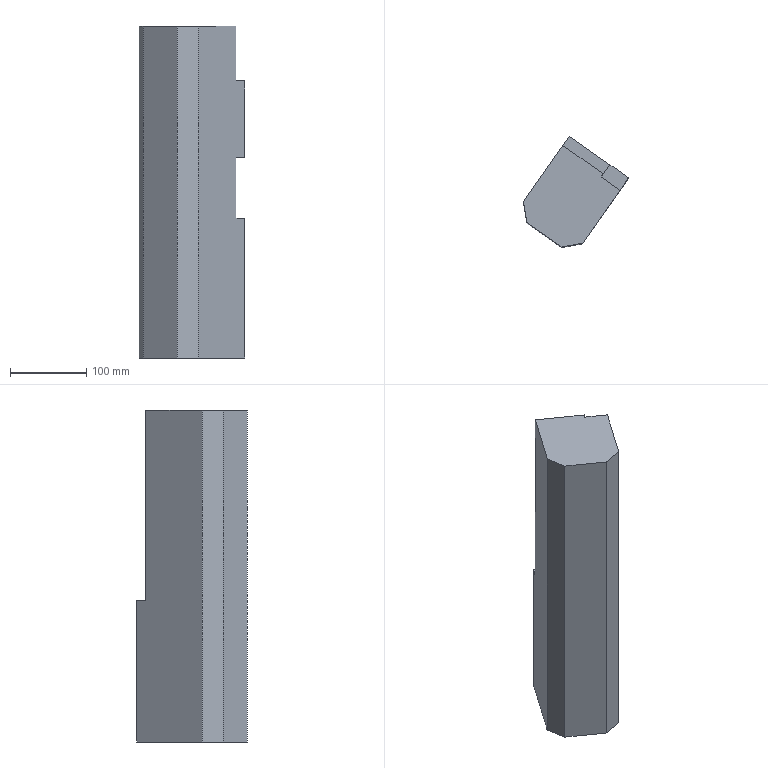Part | NX | features solid 2 | 1 solid | 19 faces | box 138.045 x 145.412 x 435 mm | volume 4656663 mm3 | plane 19
STEP:
#1=CARTESIAN_POINT('',(-261.776,-225.662,-154.062));
#2=VERTEX_POINT('',#1);
#3=CARTESIAN_POINT('',(-216.723,-257.209,-154.062));
#4=VERTEX_POINT('',#3);
#5=CARTESIAN_POINT('',(-278.159,-214.19,-154.062));
#6=DIRECTION('',(0.8192,-0.5736,0.));
#7=VECTOR('',#6,1000.);
#8=LINE('',#5,#7);
#9=EDGE_CURVE('',#2,#4,#8,.T.);
#10=ORIENTED_EDGE('',*,*,#9,.T.);
#11=CARTESIAN_POINT('',(-188.868,-252.297,-154.062));
#12=VERTEX_POINT('',#11);
#13=CARTESIAN_POINT('',(-188.868,-252.297,-154.062));
#14=DIRECTION('',(0.9848,0.1736,0.));
#15=VECTOR('',#14,1000.);
#16=LINE('',#13,#15);
#17=EDGE_CURVE('',#4,#12,#16,.T.);
#18=ORIENTED_EDGE('',*,*,#17,.T.);
#19=CARTESIAN_POINT('',(-140.114,-182.669,-154.062));
#20=VERTEX_POINT('',#19);
#21=CARTESIAN_POINT('',(-48.342,-51.605,-154.062));
#22=DIRECTION('',(0.5736,0.8192,0.));
#23=VECTOR('',#22,1000.);
#24=LINE('',#21,#23);
#25=EDGE_CURVE('',#20,#12,#24,.F.);
#26=ORIENTED_EDGE('',*,*,#25,.F.);
#27=CARTESIAN_POINT('',(-164.689,-165.462,-154.062));
#28=VERTEX_POINT('',#27);
#29=CARTESIAN_POINT('',(-217.934,-128.179,-154.062));
#30=DIRECTION('',(0.8192,-0.5736,0.));
#31=VECTOR('',#30,1000.);
#32=LINE('',#29,#31);
#33=EDGE_CURVE('',#28,#20,#32,.T.);
#34=ORIENTED_EDGE('',*,*,#33,.F.);
#35=CARTESIAN_POINT('',(-161.821,-161.366,-154.062));
#36=VERTEX_POINT('',#35);
#37=CARTESIAN_POINT('',(-161.821,-161.366,-154.062));
#38=DIRECTION('',(0.5736,0.8192,0.));
#39=VECTOR('',#38,1000.);
#40=LINE('',#37,#39);
#41=EDGE_CURVE('',#28,#36,#40,.T.);
#42=ORIENTED_EDGE('',*,*,#41,.T.);
#43=CARTESIAN_POINT('',(-215.066,-124.084,-154.062));
#44=VERTEX_POINT('',#43);
#45=CARTESIAN_POINT('',(-215.066,-124.084,-154.062));
#46=DIRECTION('',(0.8192,-0.5736,0.));
#47=VECTOR('',#46,1000.);
#48=LINE('',#45,#47);
#49=EDGE_CURVE('',#44,#36,#48,.T.);
#50=ORIENTED_EDGE('',*,*,#49,.F.);
#51=CARTESIAN_POINT('',(-266.688,-197.807,-154.062));
#52=VERTEX_POINT('',#51);
#53=CARTESIAN_POINT('',(-215.066,-124.084,-154.062));
#54=DIRECTION('',(-0.5736,-0.8192,0.));
#55=VECTOR('',#54,1000.);
#56=LINE('',#53,#55);
#57=EDGE_CURVE('',#44,#52,#56,.T.);
#58=ORIENTED_EDGE('',*,*,#57,.T.);
#59=CARTESIAN_POINT('',(-261.776,-225.662,-154.062));
#60=DIRECTION('',(0.1736,-0.9848,0.));
#61=VECTOR('',#60,1000.);
#62=LINE('',#59,#61);
#63=EDGE_CURVE('',#52,#2,#62,.T.);
#64=ORIENTED_EDGE('',*,*,#63,.T.);
#65=EDGE_LOOP('',(#10,#18,#26,#34,#42,#50,#58,#64));
#66=FACE_BOUND('',#65,.T.);
#67=CARTESIAN_POINT('',(-215.066,-124.084,-154.062));
#68=DIRECTION('',(0.,0.,-1.));
#69=DIRECTION('',(-0.5736,-0.8192,0.));
#70=AXIS2_PLACEMENT_3D('',#67,#68,#69);
#71=PLANE('',#70);
#72=ADVANCED_FACE('',(#66),#71,.F.);
#73=CARTESIAN_POINT('',(-161.821,-161.366,-226.082));
#74=VERTEX_POINT('',#73);
#75=CARTESIAN_POINT('',(-161.821,-161.366,-326.082));
#76=VERTEX_POINT('',#75);
#77=CARTESIAN_POINT('',(-161.821,-161.366,-401.082));
#78=DIRECTION('',(0.,0.,-1.));
#79=VECTOR('',#78,1000.);
#80=LINE('',#77,#79);
#81=EDGE_CURVE('',#74,#76,#80,.T.);
#82=ORIENTED_EDGE('',*,*,#81,.T.);
#83=CARTESIAN_POINT('',(-161.821,-161.366,-404.062));
#84=VERTEX_POINT('',#83);
#85=CARTESIAN_POINT('',(-161.821,-161.366,-401.082));
#86=DIRECTION('',(0.,0.,-1.));
#87=VECTOR('',#86,1000.);
#88=LINE('',#85,#87);
#89=EDGE_CURVE('',#76,#84,#88,.T.);
#90=ORIENTED_EDGE('',*,*,#89,.T.);
#91=CARTESIAN_POINT('',(-215.066,-124.084,-404.062));
#92=VERTEX_POINT('',#91);
#93=CARTESIAN_POINT('',(-215.066,-124.084,-404.062));
#94=DIRECTION('',(-0.8192,0.5736,0.));
#95=VECTOR('',#94,1000.);
#96=LINE('',#93,#95);
#97=EDGE_CURVE('',#84,#92,#96,.T.);
#98=ORIENTED_EDGE('',*,*,#97,.T.);
#99=CARTESIAN_POINT('',(-215.066,-124.084,-401.082));
#100=DIRECTION('',(0.,0.,-1.));
#101=VECTOR('',#100,1000.);
#102=LINE('',#99,#101);
#103=EDGE_CURVE('',#44,#92,#102,.T.);
#104=ORIENTED_EDGE('',*,*,#103,.F.);
#105=ORIENTED_EDGE('',*,*,#49,.T.);
#106=CARTESIAN_POINT('',(-161.821,-161.366,-401.082));
#107=DIRECTION('',(0.,0.,1.));
#108=VECTOR('',#107,1000.);
#109=LINE('',#106,#108);
#110=EDGE_CURVE('',#74,#36,#109,.T.);
#111=ORIENTED_EDGE('',*,*,#110,.F.);
#112=EDGE_LOOP('',(#82,#90,#98,#104,#105,#111));
#113=FACE_BOUND('',#112,.T.);
#114=CARTESIAN_POINT('',(-215.066,-124.084,-401.082));
#115=DIRECTION('',(-0.5736,-0.8192,0.));
#116=DIRECTION('',(0.8192,-0.5736,0.));
#117=AXIS2_PLACEMENT_3D('',#114,#115,#116);
#118=PLANE('',#117);
#119=ADVANCED_FACE('',(#113),#118,.F.);
#120=CARTESIAN_POINT('',(-153.217,-149.079,-404.062));
#121=VERTEX_POINT('',#120);
#122=CARTESIAN_POINT('',(-153.217,-149.079,-406.082));
#123=VERTEX_POINT('',#122);
#124=CARTESIAN_POINT('',(-153.217,-149.079,-326.082));
#125=DIRECTION('',(0.,0.,-1.));
#126=VECTOR('',#125,1000.);
#127=LINE('',#124,#126);
#128=EDGE_CURVE('',#121,#123,#127,.T.);
#129=ORIENTED_EDGE('',*,*,#128,.T.);
#130=CARTESIAN_POINT('',(-128.643,-166.286,-406.082));
#131=VERTEX_POINT('',#130);
#132=CARTESIAN_POINT('',(-153.217,-149.079,-406.082));
#133=DIRECTION('',(0.8192,-0.5736,0.));
#134=VECTOR('',#133,1000.);
#135=LINE('',#132,#134);
#136=EDGE_CURVE('',#123,#131,#135,.T.);
#137=ORIENTED_EDGE('',*,*,#136,.T.);
#138=CARTESIAN_POINT('',(-128.643,-166.286,-589.062));
#139=VERTEX_POINT('',#138);
#140=CARTESIAN_POINT('',(-128.643,-166.286,-400.));
#141=DIRECTION('',(0.,0.,1.));
#142=VECTOR('',#141,1000.);
#143=LINE('',#140,#142);
#144=EDGE_CURVE('',#131,#139,#143,.F.);
#145=ORIENTED_EDGE('',*,*,#144,.T.);
#146=CARTESIAN_POINT('',(-206.462,-111.796,-589.062));
#147=VERTEX_POINT('',#146);
#148=CARTESIAN_POINT('',(-206.544,-111.739,-589.062));
#149=DIRECTION('',(0.8192,-0.5736,0.));
#150=VECTOR('',#149,1000.);
#151=LINE('',#148,#150);
#152=EDGE_CURVE('',#139,#147,#151,.F.);
#153=ORIENTED_EDGE('',*,*,#152,.T.);
#154=CARTESIAN_POINT('',(-206.462,-111.796,-404.062));
#155=VERTEX_POINT('',#154);
#156=CARTESIAN_POINT('',(-206.462,-111.796,-401.082));
#157=DIRECTION('',(0.,0.,-1.));
#158=VECTOR('',#157,1000.);
#159=LINE('',#156,#158);
#160=EDGE_CURVE('',#155,#147,#159,.T.);
#161=ORIENTED_EDGE('',*,*,#160,.F.);
#162=CARTESIAN_POINT('',(-153.217,-149.079,-404.062));
#163=DIRECTION('',(-0.8192,0.5736,0.));
#164=VECTOR('',#163,1000.);
#165=LINE('',#162,#164);
#166=EDGE_CURVE('',#121,#155,#165,.T.);
#167=ORIENTED_EDGE('',*,*,#166,.F.);
#168=EDGE_LOOP('',(#129,#137,#145,#153,#161,#167));
#169=FACE_BOUND('',#168,.T.);
#170=CARTESIAN_POINT('',(-153.217,-149.079,-461.082));
#171=DIRECTION('',(0.5736,0.8192,0.));
#172=DIRECTION('',(-0.8192,0.5736,0.));
#173=AXIS2_PLACEMENT_3D('',#170,#171,#172);
#174=PLANE('',#173);
#175=ADVANCED_FACE('',(#169),#174,.T.);
#176=CARTESIAN_POINT('',(-188.868,-252.297,-589.062));
#177=VERTEX_POINT('',#176);
#178=CARTESIAN_POINT('',(-197.472,-264.584,-589.062));
#179=DIRECTION('',(-0.5736,-0.8192,0.));
#180=VECTOR('',#179,1000.);
#181=LINE('',#178,#180);
#182=EDGE_CURVE('',#139,#177,#181,.T.);
#183=ORIENTED_EDGE('',*,*,#182,.T.);
#184=CARTESIAN_POINT('',(-216.723,-257.209,-589.062));
#185=VERTEX_POINT('',#184);
#186=CARTESIAN_POINT('',(-188.868,-252.297,-589.062));
#187=DIRECTION('',(0.9848,0.1736,0.));
#188=VECTOR('',#187,1000.);
#189=LINE('',#186,#188);
#190=EDGE_CURVE('',#177,#185,#189,.F.);
#191=ORIENTED_EDGE('',*,*,#190,.T.);
#192=CARTESIAN_POINT('',(-261.776,-225.662,-589.062));
#193=VERTEX_POINT('',#192);
#194=CARTESIAN_POINT('',(-278.241,-214.133,-589.062));
#195=DIRECTION('',(0.8192,-0.5736,0.));
#196=VECTOR('',#195,1000.);
#197=LINE('',#194,#196);
#198=EDGE_CURVE('',#185,#193,#197,.F.);
#199=ORIENTED_EDGE('',*,*,#198,.T.);
#200=CARTESIAN_POINT('',(-266.688,-197.807,-589.062));
#201=VERTEX_POINT('',#200);
#202=CARTESIAN_POINT('',(-261.776,-225.662,-589.062));
#203=DIRECTION('',(0.1736,-0.9848,0.));
#204=VECTOR('',#203,1000.);
#205=LINE('',#202,#204);
#206=EDGE_CURVE('',#193,#201,#205,.F.);
#207=ORIENTED_EDGE('',*,*,#206,.T.);
#208=CARTESIAN_POINT('',(-275.291,-210.095,-589.062));
#209=DIRECTION('',(0.5736,0.8192,0.));
#210=VECTOR('',#209,1000.);
#211=LINE('',#208,#210);
#212=EDGE_CURVE('',#147,#201,#211,.F.);
#213=ORIENTED_EDGE('',*,*,#212,.F.);
#214=ORIENTED_EDGE('',*,*,#152,.F.);
#215=EDGE_LOOP('',(#183,#191,#199,#207,#213,#214));
#216=FACE_BOUND('',#215,.T.);
#217=CARTESIAN_POINT('',(-275.373,-210.037,-589.062));
#218=DIRECTION('',(0.,0.,-1.));
#219=DIRECTION('',(0.5736,0.8192,0.));
#220=AXIS2_PLACEMENT_3D('',#217,#218,#219);
#221=PLANE('',#220);
#222=ADVANCED_FACE('',(#216),#221,.T.);
#223=ORIENTED_EDGE('',*,*,#212,.T.);
#224=CARTESIAN_POINT('',(-266.688,-197.807,-151.082));
#225=DIRECTION('',(0.,0.,1.));
#226=VECTOR('',#225,1000.);
#227=LINE('',#224,#226);
#228=EDGE_CURVE('',#201,#52,#227,.T.);
#229=ORIENTED_EDGE('',*,*,#228,.T.);
#230=ORIENTED_EDGE('',*,*,#57,.F.);
#231=ORIENTED_EDGE('',*,*,#103,.T.);
#232=CARTESIAN_POINT('',(-215.066,-124.084,-404.062));
#233=DIRECTION('',(-0.5736,-0.8192,0.));
#234=VECTOR('',#233,1000.);
#235=LINE('',#232,#234);
#236=EDGE_CURVE('',#155,#92,#235,.T.);
#237=ORIENTED_EDGE('',*,*,#236,.F.);
#238=ORIENTED_EDGE('',*,*,#160,.T.);
#239=EDGE_LOOP('',(#223,#229,#230,#231,#237,#238));
#240=FACE_BOUND('',#239,.T.);
#241=CARTESIAN_POINT('',(-215.066,-124.084,-151.082));
#242=DIRECTION('',(-0.8192,0.5736,0.));
#243=DIRECTION('',(-0.5736,-0.8192,0.));
#244=AXIS2_PLACEMENT_3D('',#241,#242,#243);
#245=PLANE('',#244);
#246=ADVANCED_FACE('',(#240),#245,.T.);
#247=ORIENTED_EDGE('',*,*,#198,.F.);
#248=CARTESIAN_POINT('',(-216.723,-257.209,-192.696));
#249=DIRECTION('',(0.,0.,1.));
#250=VECTOR('',#249,1000.);
#251=LINE('',#248,#250);
#252=EDGE_CURVE('',#185,#4,#251,.T.);
#253=ORIENTED_EDGE('',*,*,#252,.T.);
#254=ORIENTED_EDGE('',*,*,#9,.F.);
#255=CARTESIAN_POINT('',(-261.776,-225.662,-589.062));
#256=DIRECTION('',(0.,0.,-1.));
#257=VECTOR('',#256,1000.);
#258=LINE('',#255,#257);
#259=EDGE_CURVE('',#2,#193,#258,.T.);
#260=ORIENTED_EDGE('',*,*,#259,.T.);
#261=EDGE_LOOP('',(#247,#253,#254,#260));
#262=FACE_BOUND('',#261,.T.);
#263=CARTESIAN_POINT('',(-789.915,144.145,-192.696));
#264=DIRECTION('',(0.5736,0.8192,0.));
#265=DIRECTION('',(-0.8192,0.5736,0.));
#266=AXIS2_PLACEMENT_3D('',#263,#264,#265);
#267=PLANE('',#266);
#268=ADVANCED_FACE('',(#262),#267,.F.);
#269=CARTESIAN_POINT('',(-161.821,-161.366,-404.062));
#270=DIRECTION('',(-0.5736,-0.8192,0.));
#271=VECTOR('',#270,1000.);
#272=LINE('',#269,#271);
#273=EDGE_CURVE('',#121,#84,#272,.T.);
#274=ORIENTED_EDGE('',*,*,#273,.F.);
#275=ORIENTED_EDGE('',*,*,#166,.T.);
#276=ORIENTED_EDGE('',*,*,#236,.T.);
#277=ORIENTED_EDGE('',*,*,#97,.F.);
#278=EDGE_LOOP('',(#274,#275,#276,#277));
#279=FACE_BOUND('',#278,.T.);
#280=CARTESIAN_POINT('',(-161.821,-161.366,-404.062));
#281=DIRECTION('',(0.,0.,1.));
#282=DIRECTION('',(0.5736,0.8192,0.));
#283=AXIS2_PLACEMENT_3D('',#280,#281,#282);
#284=PLANE('',#283);
#285=ADVANCED_FACE('',(#279),#284,.T.);
#286=CARTESIAN_POINT('',(-140.114,-182.669,-326.082));
#287=VERTEX_POINT('',#286);
#288=CARTESIAN_POINT('',(-128.643,-166.286,-326.082));
#289=VERTEX_POINT('',#288);
#290=CARTESIAN_POINT('',(-137.246,-178.573,-326.082));
#291=DIRECTION('',(-0.5736,-0.8192,0.));
#292=VECTOR('',#291,1000.);
#293=LINE('',#290,#292);
#294=EDGE_CURVE('',#287,#289,#293,.F.);
#295=ORIENTED_EDGE('',*,*,#294,.F.);
#296=CARTESIAN_POINT('',(-164.689,-165.462,-326.082));
#297=VERTEX_POINT('',#296);
#298=CARTESIAN_POINT('',(-164.689,-165.462,-326.082));
#299=DIRECTION('',(0.8192,-0.5736,0.));
#300=VECTOR('',#299,1000.);
#301=LINE('',#298,#300);
#302=EDGE_CURVE('',#297,#287,#301,.T.);
#303=ORIENTED_EDGE('',*,*,#302,.F.);
#304=CARTESIAN_POINT('',(-161.821,-161.366,-326.082));
#305=DIRECTION('',(0.5736,0.8192,0.));
#306=VECTOR('',#305,1000.);
#307=LINE('',#304,#306);
#308=EDGE_CURVE('',#297,#76,#307,.T.);
#309=ORIENTED_EDGE('',*,*,#308,.T.);
#310=CARTESIAN_POINT('',(-153.217,-149.079,-326.082));
#311=VERTEX_POINT('',#310);
#312=CARTESIAN_POINT('',(-161.821,-161.366,-326.082));
#313=DIRECTION('',(0.5736,0.8192,0.));
#314=VECTOR('',#313,1000.);
#315=LINE('',#312,#314);
#316=EDGE_CURVE('',#76,#311,#315,.T.);
#317=ORIENTED_EDGE('',*,*,#316,.T.);
#318=CARTESIAN_POINT('',(-153.217,-149.079,-326.082));
#319=DIRECTION('',(-0.8192,0.5736,0.));
#320=VECTOR('',#319,1000.);
#321=LINE('',#318,#320);
#322=EDGE_CURVE('',#311,#289,#321,.F.);
#323=ORIENTED_EDGE('',*,*,#322,.T.);
#324=EDGE_LOOP('',(#295,#303,#309,#317,#323));
#325=FACE_BOUND('',#324,.T.);
#326=CARTESIAN_POINT('',(-161.821,-161.366,-326.082));
#327=DIRECTION('',(0.,0.,-1.));
#328=DIRECTION('',(-0.9063,-0.4226,0.));
#329=AXIS2_PLACEMENT_3D('',#326,#327,#328);
#330=PLANE('',#329);
#331=ADVANCED_FACE('',(#325),#330,.T.);
#332=CARTESIAN_POINT('',(-164.689,-165.462,-226.082));
#333=VERTEX_POINT('',#332);
#334=CARTESIAN_POINT('',(-140.114,-182.669,-226.082));
#335=VERTEX_POINT('',#334);
#336=CARTESIAN_POINT('',(-217.934,-128.179,-226.082));
#337=DIRECTION('',(0.8192,-0.5736,0.));
#338=VECTOR('',#337,1000.);
#339=LINE('',#336,#338);
#340=EDGE_CURVE('',#333,#335,#339,.T.);
#341=ORIENTED_EDGE('',*,*,#340,.T.);
#342=CARTESIAN_POINT('',(-128.643,-166.286,-226.082));
#343=VERTEX_POINT('',#342);
#344=CARTESIAN_POINT('',(-137.246,-178.573,-226.082));
#345=DIRECTION('',(-0.5736,-0.8192,0.));
#346=VECTOR('',#345,1000.);
#347=LINE('',#344,#346);
#348=EDGE_CURVE('',#335,#343,#347,.F.);
#349=ORIENTED_EDGE('',*,*,#348,.T.);
#350=CARTESIAN_POINT('',(-153.217,-149.079,-226.082));
#351=VERTEX_POINT('',#350);
#352=CARTESIAN_POINT('',(-153.217,-149.079,-226.082));
#353=DIRECTION('',(-0.8192,0.5736,0.));
#354=VECTOR('',#353,1000.);
#355=LINE('',#352,#354);
#356=EDGE_CURVE('',#351,#343,#355,.F.);
#357=ORIENTED_EDGE('',*,*,#356,.F.);
#358=CARTESIAN_POINT('',(-161.821,-161.366,-226.082));
#359=DIRECTION('',(0.5736,0.8192,0.));
#360=VECTOR('',#359,1000.);
#361=LINE('',#358,#360);
#362=EDGE_CURVE('',#74,#351,#361,.T.);
#363=ORIENTED_EDGE('',*,*,#362,.F.);
#364=CARTESIAN_POINT('',(-161.821,-161.366,-226.082));
#365=DIRECTION('',(0.5736,0.8192,0.));
#366=VECTOR('',#365,1000.);
#367=LINE('',#364,#366);
#368=EDGE_CURVE('',#333,#74,#367,.T.);
#369=ORIENTED_EDGE('',*,*,#368,.F.);
#370=EDGE_LOOP('',(#341,#349,#357,#363,#369));
#371=FACE_BOUND('',#370,.T.);
#372=CARTESIAN_POINT('',(-161.821,-161.366,-226.082));
#373=DIRECTION('',(0.,0.,-1.));
#374=DIRECTION('',(-0.9063,-0.4226,0.));
#375=AXIS2_PLACEMENT_3D('',#372,#373,#374);
#376=PLANE('',#375);
#377=ADVANCED_FACE('',(#371),#376,.F.);
#378=ORIENTED_EDGE('',*,*,#81,.F.);
#379=ORIENTED_EDGE('',*,*,#362,.T.);
#380=CARTESIAN_POINT('',(-153.217,-149.079,-461.082));
#381=DIRECTION('',(0.,0.,1.));
#382=VECTOR('',#381,1000.);
#383=LINE('',#380,#382);
#384=EDGE_CURVE('',#351,#311,#383,.F.);
#385=ORIENTED_EDGE('',*,*,#384,.T.);
#386=ORIENTED_EDGE('',*,*,#316,.F.);
#387=EDGE_LOOP('',(#378,#379,#385,#386));
#388=FACE_BOUND('',#387,.T.);
#389=CARTESIAN_POINT('',(-161.821,-161.366,-151.082));
#390=DIRECTION('',(-0.8192,0.5736,0.));
#391=DIRECTION('',(-0.5736,-0.8192,0.));
#392=AXIS2_PLACEMENT_3D('',#389,#390,#391);
#393=PLANE('',#392);
#394=ADVANCED_FACE('',(#388),#393,.T.);
#395=CARTESIAN_POINT('',(-128.643,-166.286,-461.082));
#396=DIRECTION('',(0.,0.,-1.));
#397=VECTOR('',#396,1000.);
#398=LINE('',#395,#397);
#399=EDGE_CURVE('',#343,#289,#398,.T.);
#400=ORIENTED_EDGE('',*,*,#399,.T.);
#401=ORIENTED_EDGE('',*,*,#322,.F.);
#402=ORIENTED_EDGE('',*,*,#384,.F.);
#403=ORIENTED_EDGE('',*,*,#356,.T.);
#404=EDGE_LOOP('',(#400,#401,#402,#403));
#405=FACE_BOUND('',#404,.T.);
#406=CARTESIAN_POINT('',(-153.217,-149.079,-461.082));
#407=DIRECTION('',(0.5736,0.8192,0.));
#408=DIRECTION('',(-0.8192,0.5736,0.));
#409=AXIS2_PLACEMENT_3D('',#406,#407,#408);
#410=PLANE('',#409);
#411=ADVANCED_FACE('',(#405),#410,.T.);
#412=ORIENTED_EDGE('',*,*,#25,.T.);
#413=CARTESIAN_POINT('',(-188.868,-252.297,-400.));
#414=DIRECTION('',(0.,0.,1.));
#415=VECTOR('',#414,1000.);
#416=LINE('',#413,#415);
#417=EDGE_CURVE('',#12,#177,#416,.F.);
#418=ORIENTED_EDGE('',*,*,#417,.T.);
#419=ORIENTED_EDGE('',*,*,#182,.F.);
#420=ORIENTED_EDGE('',*,*,#144,.F.);
#421=CARTESIAN_POINT('',(-140.114,-182.669,-406.082));
#422=VERTEX_POINT('',#421);
#423=CARTESIAN_POINT('',(-48.342,-51.605,-406.082));
#424=DIRECTION('',(0.5736,0.8192,0.));
#425=VECTOR('',#424,1000.);
#426=LINE('',#423,#425);
#427=EDGE_CURVE('',#131,#422,#426,.F.);
#428=ORIENTED_EDGE('',*,*,#427,.T.);
#429=CARTESIAN_POINT('',(-140.114,-182.669,-400.));
#430=DIRECTION('',(0.,0.,1.));
#431=VECTOR('',#430,1000.);
#432=LINE('',#429,#431);
#433=EDGE_CURVE('',#287,#422,#432,.F.);
#434=ORIENTED_EDGE('',*,*,#433,.F.);
#435=ORIENTED_EDGE('',*,*,#294,.T.);
#436=ORIENTED_EDGE('',*,*,#399,.F.);
#437=ORIENTED_EDGE('',*,*,#348,.F.);
#438=CARTESIAN_POINT('',(-140.114,-182.669,-400.));
#439=DIRECTION('',(0.,0.,-1.));
#440=VECTOR('',#439,1000.);
#441=LINE('',#438,#440);
#442=EDGE_CURVE('',#335,#20,#441,.F.);
#443=ORIENTED_EDGE('',*,*,#442,.T.);
#444=EDGE_LOOP('',(#412,#418,#419,#420,#428,#434,#435,#436,#437,#443));
#445=FACE_BOUND('',#444,.T.);
#446=CARTESIAN_POINT('',(-48.342,-51.605,-400.));
#447=DIRECTION('',(0.8192,-0.5736,0.));
#448=DIRECTION('',(0.,0.,1.));
#449=AXIS2_PLACEMENT_3D('',#446,#447,#448);
#450=PLANE('',#449);
#451=ADVANCED_FACE('',(#445),#450,.T.);
#452=ORIENTED_EDGE('',*,*,#110,.T.);
#453=ORIENTED_EDGE('',*,*,#41,.F.);
#454=CARTESIAN_POINT('',(-164.689,-165.462,-226.082));
#455=DIRECTION('',(0.,0.,1.));
#456=VECTOR('',#455,1000.);
#457=LINE('',#454,#456);
#458=EDGE_CURVE('',#333,#28,#457,.T.);
#459=ORIENTED_EDGE('',*,*,#458,.F.);
#460=ORIENTED_EDGE('',*,*,#368,.T.);
#461=EDGE_LOOP('',(#452,#453,#459,#460));
#462=FACE_BOUND('',#461,.T.);
#463=CARTESIAN_POINT('',(-161.821,-161.366,-226.082));
#464=DIRECTION('',(0.8192,-0.5736,0.));
#465=DIRECTION('',(0.5736,0.8192,0.));
#466=AXIS2_PLACEMENT_3D('',#463,#464,#465);
#467=PLANE('',#466);
#468=ADVANCED_FACE('',(#462),#467,.T.);
#469=ORIENTED_EDGE('',*,*,#33,.T.);
#470=ORIENTED_EDGE('',*,*,#442,.F.);
#471=ORIENTED_EDGE('',*,*,#340,.F.);
#472=ORIENTED_EDGE('',*,*,#458,.T.);
#473=EDGE_LOOP('',(#469,#470,#471,#472));
#474=FACE_BOUND('',#473,.T.);
#475=CARTESIAN_POINT('',(-217.934,-128.179,-226.082));
#476=DIRECTION('',(-0.5736,-0.8192,0.));
#477=DIRECTION('',(0.8192,-0.5736,0.));
#478=AXIS2_PLACEMENT_3D('',#475,#476,#477);
#479=PLANE('',#478);
#480=ADVANCED_FACE('',(#474),#479,.F.);
#481=ORIENTED_EDGE('',*,*,#136,.F.);
#482=CARTESIAN_POINT('',(-164.689,-165.462,-406.082));
#483=VERTEX_POINT('',#482);
#484=CARTESIAN_POINT('',(-161.821,-161.366,-406.082));
#485=DIRECTION('',(0.5736,0.8192,0.));
#486=VECTOR('',#485,1000.);
#487=LINE('',#484,#486);
#488=EDGE_CURVE('',#483,#123,#487,.T.);
#489=ORIENTED_EDGE('',*,*,#488,.F.);
#490=CARTESIAN_POINT('',(-164.689,-165.462,-406.082));
#491=DIRECTION('',(0.8192,-0.5736,0.));
#492=VECTOR('',#491,1000.);
#493=LINE('',#490,#492);
#494=EDGE_CURVE('',#483,#422,#493,.T.);
#495=ORIENTED_EDGE('',*,*,#494,.T.);
#496=ORIENTED_EDGE('',*,*,#427,.F.);
#497=EDGE_LOOP('',(#481,#489,#495,#496));
#498=FACE_BOUND('',#497,.T.);
#499=CARTESIAN_POINT('',(-161.821,-161.366,-406.082));
#500=DIRECTION('',(0.,0.,-1.));
#501=DIRECTION('',(-0.9063,-0.4226,0.));
#502=AXIS2_PLACEMENT_3D('',#499,#500,#501);
#503=PLANE('',#502);
#504=ADVANCED_FACE('',(#498),#503,.F.);
#505=ORIENTED_EDGE('',*,*,#308,.F.);
#506=CARTESIAN_POINT('',(-164.689,-165.462,-326.082));
#507=DIRECTION('',(0.,0.,-1.));
#508=VECTOR('',#507,1000.);
#509=LINE('',#506,#508);
#510=EDGE_CURVE('',#297,#483,#509,.T.);
#511=ORIENTED_EDGE('',*,*,#510,.T.);
#512=ORIENTED_EDGE('',*,*,#488,.T.);
#513=ORIENTED_EDGE('',*,*,#128,.F.);
#514=ORIENTED_EDGE('',*,*,#273,.T.);
#515=ORIENTED_EDGE('',*,*,#89,.F.);
#516=EDGE_LOOP('',(#505,#511,#512,#513,#514,#515));
#517=FACE_BOUND('',#516,.T.);
#518=CARTESIAN_POINT('',(-161.821,-161.366,-326.082));
#519=DIRECTION('',(-0.8192,0.5736,0.));
#520=DIRECTION('',(-0.5736,-0.8192,0.));
#521=AXIS2_PLACEMENT_3D('',#518,#519,#520);
#522=PLANE('',#521);
#523=ADVANCED_FACE('',(#517),#522,.F.);
#524=ORIENTED_EDGE('',*,*,#494,.F.);
#525=ORIENTED_EDGE('',*,*,#510,.F.);
#526=ORIENTED_EDGE('',*,*,#302,.T.);
#527=ORIENTED_EDGE('',*,*,#433,.T.);
#528=EDGE_LOOP('',(#524,#525,#526,#527));
#529=FACE_BOUND('',#528,.T.);
#530=CARTESIAN_POINT('',(-217.934,-128.179,-326.082));
#531=DIRECTION('',(0.5736,0.8192,0.));
#532=DIRECTION('',(-0.8192,0.5736,0.));
#533=AXIS2_PLACEMENT_3D('',#530,#531,#532);
#534=PLANE('',#533);
#535=ADVANCED_FACE('',(#529),#534,.T.);
#536=ORIENTED_EDGE('',*,*,#63,.F.);
#537=ORIENTED_EDGE('',*,*,#228,.F.);
#538=ORIENTED_EDGE('',*,*,#206,.F.);
#539=ORIENTED_EDGE('',*,*,#259,.F.);
#540=EDGE_LOOP('',(#536,#537,#538,#539));
#541=FACE_BOUND('',#540,.T.);
#542=CARTESIAN_POINT('',(-261.776,-225.662,-192.696));
#543=DIRECTION('',(-0.9848,-0.1736,0.));
#544=DIRECTION('',(0.1736,-0.9848,0.));
#545=AXIS2_PLACEMENT_3D('',#542,#543,#544);
#546=PLANE('',#545);
#547=ADVANCED_FACE('',(#541),#546,.T.);
#548=ORIENTED_EDGE('',*,*,#17,.F.);
#549=ORIENTED_EDGE('',*,*,#252,.F.);
#550=ORIENTED_EDGE('',*,*,#190,.F.);
#551=ORIENTED_EDGE('',*,*,#417,.F.);
#552=EDGE_LOOP('',(#548,#549,#550,#551));
#553=FACE_BOUND('',#552,.T.);
#554=CARTESIAN_POINT('',(-188.868,-252.297,-400.));
#555=DIRECTION('',(0.1736,-0.9848,0.));
#556=DIRECTION('',(0.9848,0.1736,0.));
#557=AXIS2_PLACEMENT_3D('',#554,#555,#556);
#558=PLANE('',#557);
#559=ADVANCED_FACE('',(#553),#558,.T.);
#560=CLOSED_SHELL('',(#72,#119,#175,#222,#246,#268,#285,#331,#377,#394,#411,#451,#468,#480,#504,#523,#535,#547,#559));
#561=MANIFOLD_SOLID_BREP('',#560);
#562=(LENGTH_UNIT()NAMED_UNIT(*)SI_UNIT(.MILLI.,.METRE.));
#563=UNCERTAINTY_MEASURE_WITH_UNIT(LENGTH_MEASURE(0.00001),#562,'','');
#564=(NAMED_UNIT(*)PLANE_ANGLE_UNIT()SI_UNIT($,.RADIAN.));
#565=(NAMED_UNIT(*)SI_UNIT($,.STERADIAN.)SOLID_ANGLE_UNIT());
#566=(GEOMETRIC_REPRESENTATION_CONTEXT(3)GLOBAL_UNCERTAINTY_ASSIGNED_CONTEXT((#563))GLOBAL_UNIT_ASSIGNED_CONTEXT((#562,#564,#565))REPRESENTATION_CONTEXT('',''));
#567=ADVANCED_BREP_SHAPE_REPRESENTATION('',(#561),#566);